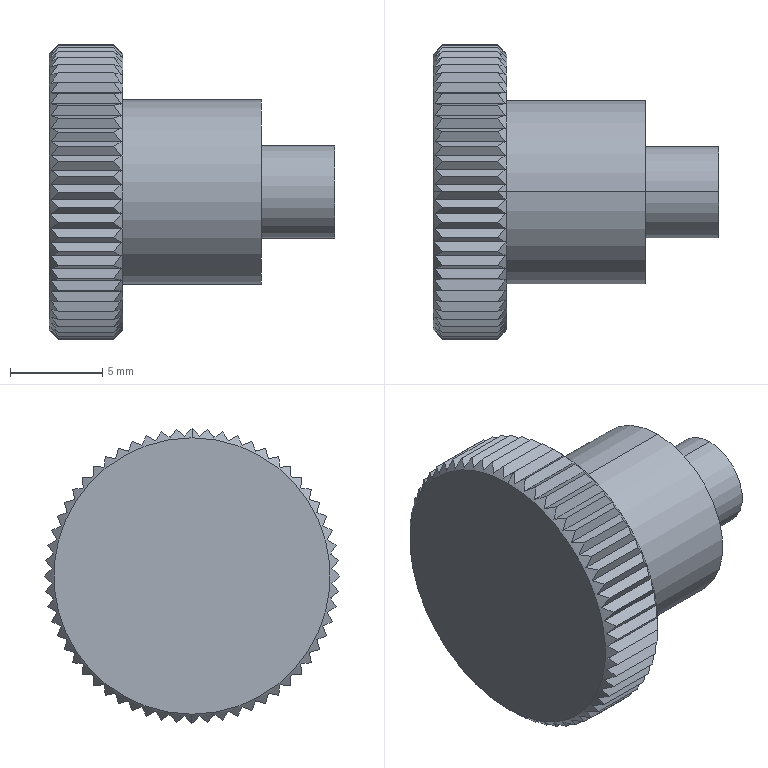Part | STEP file | 11-FG99-NKBC5_10_16-V3.0-kkkkkk-998.11_NKBC5-10-16 | 1 solid | 132 faces | box 15.5 x 16 x 16 mm | volume 1426 mm3 | plane 124 | cone 4 | cylinder 4 | commonest cylinder face diameters 5 x2 10 x2